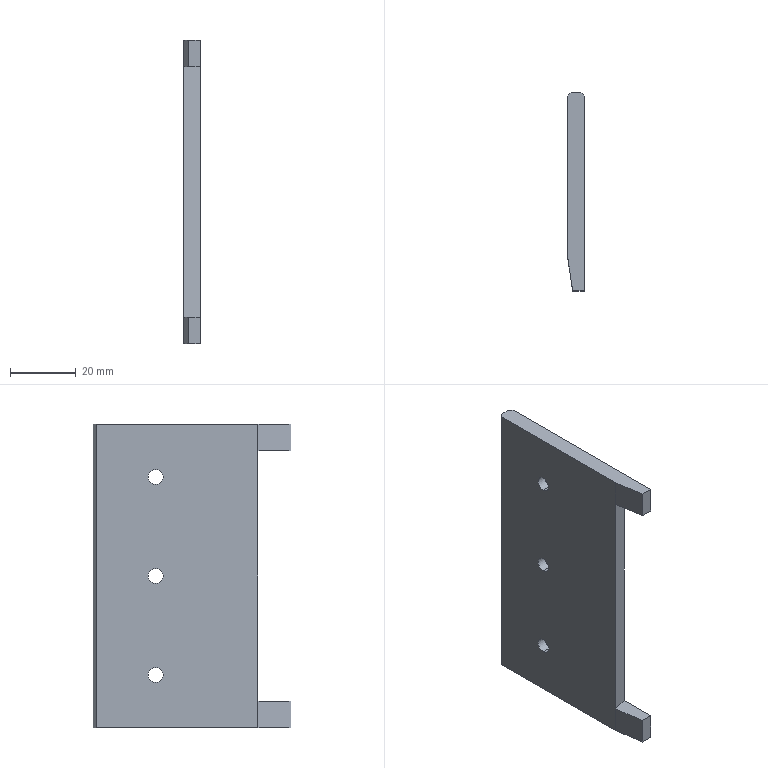Part | STEP file | 2057 Bag feed blade B | 1 solid | 26 faces | box 5 x 60 x 92 mm | volume 22979 mm3 | plane 14 | cone 6 | cylinder 6 | commonest cylinder face diameters 4.5 x6